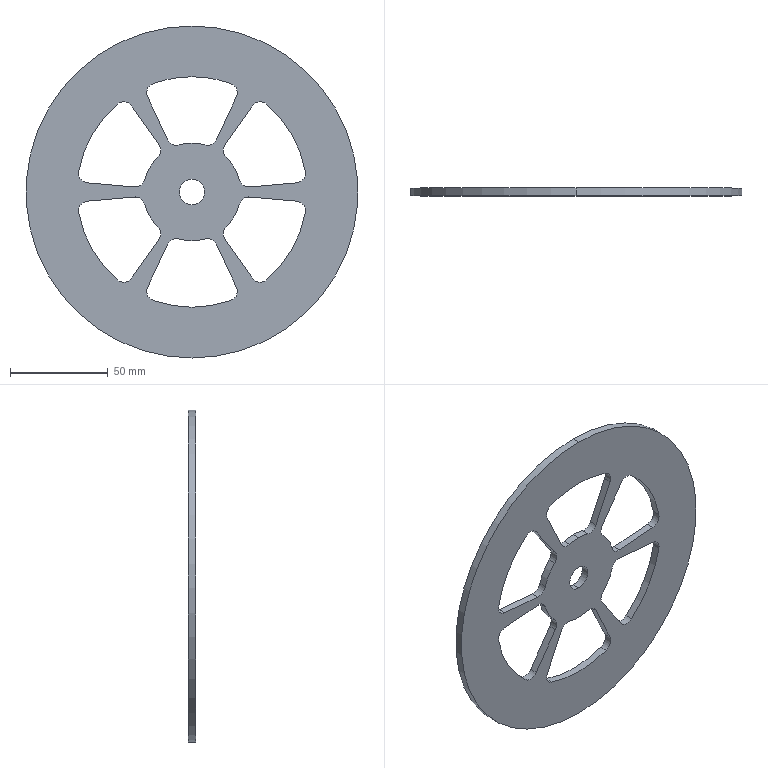Part | SolidWorks | features Extrusion 1, Fillet 1, ICE 1 | 1 solid | 62 faces | box 170 x 4 x 170 mm | volume 60845 mm3 | cylinder 48 | plane 14 | commonest cylinder face diameters 10 x30 50 x7 118 x7 13 x2 170 x2